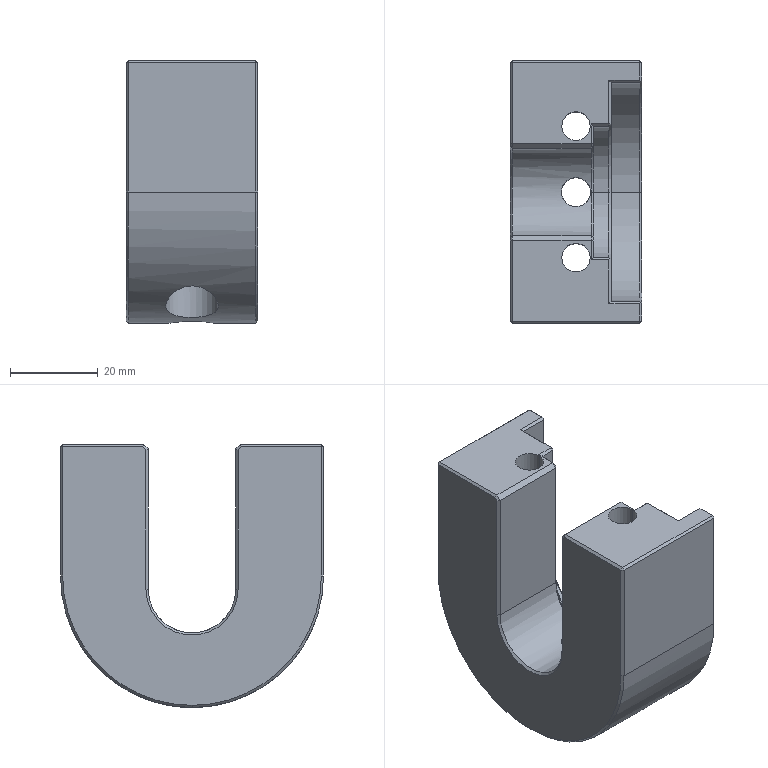Part | STEP file | PN_0013 driven wheel mounting plate_Default | 1 solid | 98 faces | box 30 x 60 x 60 mm | volume 50936 mm3 | plane 54 | cylinder 26 | cone 18 | commonest cylinder face diameters 3.3 x8 6.5 x4 12 x4 6.6 x2 11 x2 30 x2